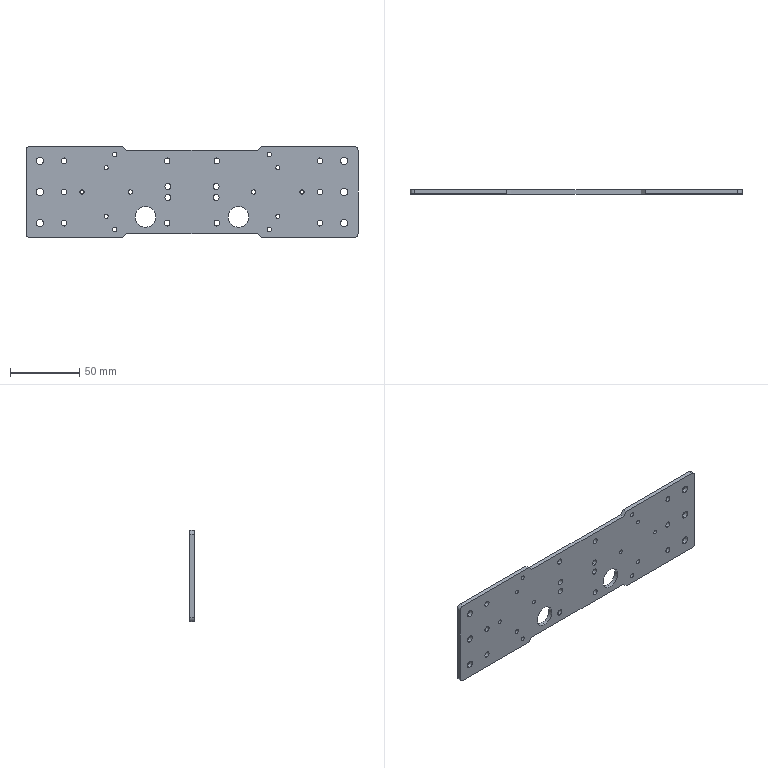Part | SolidWorks | features BaseBody 1 | 1 solid | 86 faces | box 240 x 3 x 66 mm | volume 43460 mm3 | cylinder 72 | plane 14 | commonest cylinder face diameters 4.2 x28 3 x16 5.2 x12 3.2 x8 6 x4 15 x4